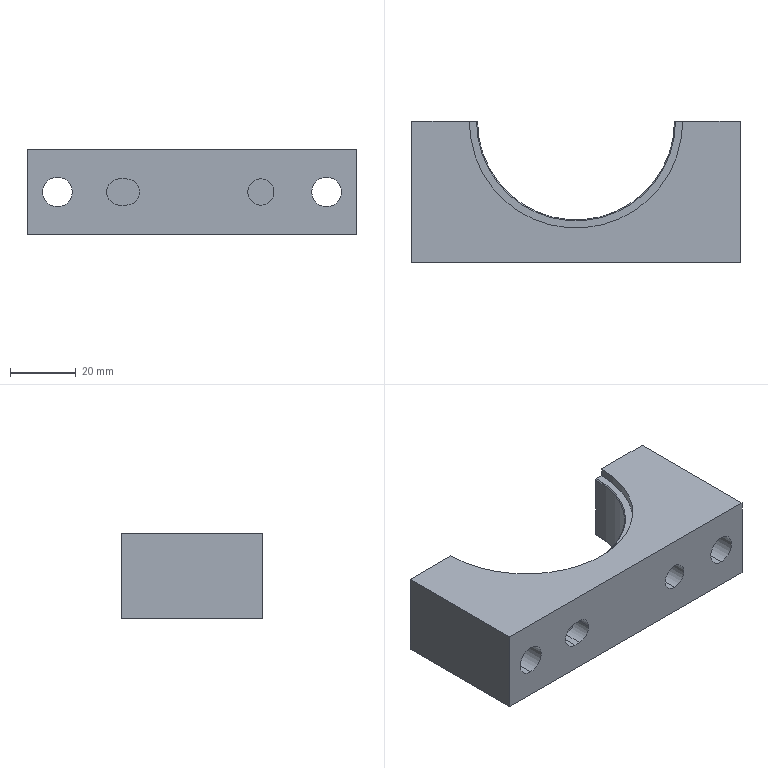Part | SolidWorks | features HoleWzd 3, ICE 3, Chamfer 1, Extrusion 1 | 1 solid | 30 faces | box 100 x 43 x 26 mm | volume 67587 mm3 | cylinder 14 | plane 14 | cone 2 | commonest cylinder face diameters 8 x5 9 x4 4 x2 65 x2 60 x1
STEP:
#1=CARTESIAN_POINT('',(-16.,-37.,13.));
#2=VERTEX_POINT('',#1);
#3=CARTESIAN_POINT('',(-20.,-37.,17.));
#4=VERTEX_POINT('',#3);
#5=CARTESIAN_POINT('',(-20.,-37.,13.));
#6=DIRECTION('',(0.,-1.,0.));
#7=DIRECTION('',(1.,0.,0.));
#8=AXIS2_PLACEMENT_3D('',#5,#6,#7);
#9=CIRCLE('',#8,4.);
#10=EDGE_CURVE('',#2,#4,#9,.T.);
#11=ORIENTED_EDGE('',*,*,#10,.F.);
#12=CARTESIAN_POINT('',(-16.,-43.,13.));
#13=VERTEX_POINT('',#12);
#14=CARTESIAN_POINT('',(-16.,-37.,13.));
#15=DIRECTION('',(0.,-1.,0.));
#16=VECTOR('',#15,1000.);
#17=LINE('',#14,#16);
#18=EDGE_CURVE('',#2,#13,#17,.T.);
#19=ORIENTED_EDGE('',*,*,#18,.T.);
#20=CARTESIAN_POINT('',(-20.,-43.,17.));
#21=VERTEX_POINT('',#20);
#22=CARTESIAN_POINT('',(-20.,-43.,13.));
#23=DIRECTION('',(0.,-1.,0.));
#24=DIRECTION('',(1.,0.,0.));
#25=AXIS2_PLACEMENT_3D('',#22,#23,#24);
#26=CIRCLE('',#25,4.);
#27=EDGE_CURVE('',#13,#21,#26,.T.);
#28=ORIENTED_EDGE('',*,*,#27,.T.);
#29=CARTESIAN_POINT('',(-20.,-37.,17.));
#30=DIRECTION('',(0.,-1.,0.));
#31=VECTOR('',#30,1000.);
#32=LINE('',#29,#31);
#33=EDGE_CURVE('',#4,#21,#32,.T.);
#34=ORIENTED_EDGE('',*,*,#33,.F.);
#35=EDGE_LOOP('',(#11,#19,#28,#34));
#36=FACE_OUTER_BOUND('',#35,.T.);
#37=CARTESIAN_POINT('',(-20.,-37.,13.));
#38=DIRECTION('',(0.,-1.,0.));
#39=DIRECTION('',(1.,0.,0.));
#40=AXIS2_PLACEMENT_3D('',#37,#38,#39);
#41=CYLINDRICAL_SURFACE('',#40,4.);
#42=ADVANCED_FACE('',(#36),#41,.F.);
#43=CARTESIAN_POINT('',(21.,-37.,17.));
#44=VERTEX_POINT('',#43);
#45=CARTESIAN_POINT('',(21.,-37.,9.));
#46=VERTEX_POINT('',#45);
#47=CARTESIAN_POINT('',(21.,-37.,13.));
#48=DIRECTION('',(0.,-1.,0.));
#49=DIRECTION('',(0.,0.,-1.));
#50=AXIS2_PLACEMENT_3D('',#47,#48,#49);
#51=CIRCLE('',#50,4.);
#52=EDGE_CURVE('',#44,#46,#51,.T.);
#53=ORIENTED_EDGE('',*,*,#52,.F.);
#54=CARTESIAN_POINT('',(21.,-43.,17.));
#55=VERTEX_POINT('',#54);
#56=CARTESIAN_POINT('',(21.,-43.,17.));
#57=DIRECTION('',(0.,-1.,0.));
#58=VECTOR('',#57,1000.);
#59=LINE('',#56,#58);
#60=EDGE_CURVE('',#44,#55,#59,.T.);
#61=ORIENTED_EDGE('',*,*,#60,.T.);
#62=CARTESIAN_POINT('',(21.,-43.,9.));
#63=VERTEX_POINT('',#62);
#64=CARTESIAN_POINT('',(21.,-43.,13.));
#65=DIRECTION('',(0.,-1.,0.));
#66=DIRECTION('',(0.,0.,-1.));
#67=AXIS2_PLACEMENT_3D('',#64,#65,#66);
#68=CIRCLE('',#67,4.);
#69=EDGE_CURVE('',#55,#63,#68,.T.);
#70=ORIENTED_EDGE('',*,*,#69,.T.);
#71=CARTESIAN_POINT('',(21.,-43.,9.));
#72=DIRECTION('',(0.,-1.,0.));
#73=VECTOR('',#72,1000.);
#74=LINE('',#71,#73);
#75=EDGE_CURVE('',#46,#63,#74,.T.);
#76=ORIENTED_EDGE('',*,*,#75,.F.);
#77=EDGE_LOOP('',(#53,#61,#70,#76));
#78=FACE_OUTER_BOUND('',#77,.T.);
#79=CARTESIAN_POINT('',(21.,-43.,13.));
#80=DIRECTION('',(0.,-1.,0.));
#81=DIRECTION('',(0.,0.,-1.));
#82=AXIS2_PLACEMENT_3D('',#79,#80,#81);
#83=CYLINDRICAL_SURFACE('',#82,4.);
#84=ADVANCED_FACE('',(#78),#83,.F.);
#85=CARTESIAN_POINT('',(0.,-34.,11.));
#86=VERTEX_POINT('',#85);
#87=CARTESIAN_POINT('',(0.,-34.,15.));
#88=VERTEX_POINT('',#87);
#89=CARTESIAN_POINT('',(0.,-34.,13.));
#90=DIRECTION('',(0.,1.,0.));
#91=DIRECTION('',(0.,0.,1.));
#92=AXIS2_PLACEMENT_3D('',#89,#90,#91);
#93=CIRCLE('',#92,2.);
#94=EDGE_CURVE('',#86,#88,#93,.T.);
#95=ORIENTED_EDGE('',*,*,#94,.F.);
#96=CARTESIAN_POINT('',(0.,-30.,11.));
#97=VERTEX_POINT('',#96);
#98=CARTESIAN_POINT('',(0.,0.,11.));
#99=DIRECTION('',(0.,1.,0.));
#100=VECTOR('',#99,1000.);
#101=LINE('',#98,#100);
#102=EDGE_CURVE('',#86,#97,#101,.T.);
#103=ORIENTED_EDGE('',*,*,#102,.T.);
#104=CARTESIAN_POINT('',(0.,-30.,15.));
#105=VERTEX_POINT('',#104);
#106=CARTESIAN_POINT('',(0.,-30.,15.));
#107=CARTESIAN_POINT('',(-0.1322,-30.,15.));
#108=CARTESIAN_POINT('',(-0.2622,-29.999,14.987));
#109=CARTESIAN_POINT('',(-0.5178,-29.996,14.936));
#110=CARTESIAN_POINT('',(-0.6449,-29.993,14.898));
#111=CARTESIAN_POINT('',(-0.8871,-29.987,14.797));
#112=CARTESIAN_POINT('',(-1.002,-29.983,14.736));
#113=CARTESIAN_POINT('',(-1.219,-29.975,14.591));
#114=CARTESIAN_POINT('',(-1.322,-29.971,14.506));
#115=CARTESIAN_POINT('',(-1.599,-29.958,14.229));
#116=CARTESIAN_POINT('',(-1.748,-29.949,14.006));
#117=CARTESIAN_POINT('',(-1.947,-29.937,13.525));
#118=CARTESIAN_POINT('',(-2.,-29.933,13.262));
#119=CARTESIAN_POINT('',(-2.,-29.933,12.87));
#120=CARTESIAN_POINT('',(-1.987,-29.934,12.738));
#121=CARTESIAN_POINT('',(-1.936,-29.937,12.481));
#122=CARTESIAN_POINT('',(-1.898,-29.94,12.356));
#123=CARTESIAN_POINT('',(-1.798,-29.946,12.114));
#124=CARTESIAN_POINT('',(-1.735,-29.95,11.997));
#125=CARTESIAN_POINT('',(-1.591,-29.958,11.78));
#126=CARTESIAN_POINT('',(-1.508,-29.962,11.679));
#127=CARTESIAN_POINT('',(-1.321,-29.971,11.493));
#128=CARTESIAN_POINT('',(-1.22,-29.975,11.41));
#129=CARTESIAN_POINT('',(-1.003,-29.983,11.265));
#130=CARTESIAN_POINT('',(-0.8865,-29.987,11.202));
#131=CARTESIAN_POINT('',(-0.6442,-29.993,11.102));
#132=CARTESIAN_POINT('',(-0.5195,-29.996,11.064));
#133=CARTESIAN_POINT('',(-0.2631,-29.999,11.013));
#134=CARTESIAN_POINT('',(-0.1305,-30.,11.));
#135=CARTESIAN_POINT('',(0.,-30.,11.));
#136=B_SPLINE_CURVE_WITH_KNOTS('',3,(#106,#107,#108,#109,#110,#111,#112,#113,#114,#115,#116,#117,#118,#119,#120,#121,#122,#123,#124,#125,#126,#127,#128,#129,#130,#131,#132,#133,#134,#135),.UNSPECIFIED.,.F.,.F.,(4,2,2,2,2,2,2,2,2,2,2,2,2,2,4),(0.,0.0003909,0.0007818,0.001173,0.001564,0.002345,0.003127,0.003518,0.003909,0.0043,0.004691,0.005082,0.005473,0.005864,0.006255),.UNSPECIFIED.);
#137=EDGE_CURVE('',#105,#97,#136,.T.);
#138=ORIENTED_EDGE('',*,*,#137,.F.);
#139=CARTESIAN_POINT('',(0.,0.,15.));
#140=DIRECTION('',(0.,1.,0.));
#141=VECTOR('',#140,1000.);
#142=LINE('',#139,#141);
#143=EDGE_CURVE('',#88,#105,#142,.T.);
#144=ORIENTED_EDGE('',*,*,#143,.F.);
#145=EDGE_LOOP('',(#95,#103,#138,#144));
#146=FACE_OUTER_BOUND('',#145,.T.);
#147=CARTESIAN_POINT('',(0.,0.,13.));
#148=DIRECTION('',(0.,1.,0.));
#149=DIRECTION('',(0.,0.,1.));
#150=AXIS2_PLACEMENT_3D('',#147,#148,#149);
#151=CYLINDRICAL_SURFACE('',#150,2.);
#152=ADVANCED_FACE('',(#146),#151,.F.);
#153=CARTESIAN_POINT('',(-41.,-43.,8.5));
#154=VERTEX_POINT('',#153);
#155=CARTESIAN_POINT('',(-41.,-43.,17.5));
#156=VERTEX_POINT('',#155);
#157=CARTESIAN_POINT('',(-41.,-43.,13.));
#158=DIRECTION('',(0.,1.,0.));
#159=DIRECTION('',(0.,0.,1.));
#160=AXIS2_PLACEMENT_3D('',#157,#158,#159);
#161=CIRCLE('',#160,4.5);
#162=EDGE_CURVE('',#154,#156,#161,.T.);
#163=ORIENTED_EDGE('',*,*,#162,.F.);
#164=CARTESIAN_POINT('',(-41.,0.,8.5));
#165=VERTEX_POINT('',#164);
#166=CARTESIAN_POINT('',(-41.,0.,8.5));
#167=DIRECTION('',(0.,1.,0.));
#168=VECTOR('',#167,1000.);
#169=LINE('',#166,#168);
#170=EDGE_CURVE('',#154,#165,#169,.T.);
#171=ORIENTED_EDGE('',*,*,#170,.T.);
#172=CARTESIAN_POINT('',(-41.,0.,17.5));
#173=VERTEX_POINT('',#172);
#174=CARTESIAN_POINT('',(-41.,0.,13.));
#175=DIRECTION('',(0.,1.,0.));
#176=DIRECTION('',(0.,0.,1.));
#177=AXIS2_PLACEMENT_3D('',#174,#175,#176);
#178=CIRCLE('',#177,4.5);
#179=EDGE_CURVE('',#165,#173,#178,.T.);
#180=ORIENTED_EDGE('',*,*,#179,.T.);
#181=CARTESIAN_POINT('',(-41.,0.,17.5));
#182=DIRECTION('',(0.,1.,0.));
#183=VECTOR('',#182,1000.);
#184=LINE('',#181,#183);
#185=EDGE_CURVE('',#156,#173,#184,.T.);
#186=ORIENTED_EDGE('',*,*,#185,.F.);
#187=EDGE_LOOP('',(#163,#171,#180,#186));
#188=FACE_OUTER_BOUND('',#187,.T.);
#189=CARTESIAN_POINT('',(-41.,0.,13.));
#190=DIRECTION('',(0.,1.,0.));
#191=DIRECTION('',(0.,0.,1.));
#192=AXIS2_PLACEMENT_3D('',#189,#190,#191);
#193=CYLINDRICAL_SURFACE('',#192,4.5);
#194=ADVANCED_FACE('',(#188),#193,.F.);
#195=CARTESIAN_POINT('',(41.,-43.,8.5));
#196=VERTEX_POINT('',#195);
#197=CARTESIAN_POINT('',(41.,-43.,17.5));
#198=VERTEX_POINT('',#197);
#199=CARTESIAN_POINT('',(41.,-43.,13.));
#200=DIRECTION('',(0.,1.,0.));
#201=DIRECTION('',(0.,0.,1.));
#202=AXIS2_PLACEMENT_3D('',#199,#200,#201);
#203=CIRCLE('',#202,4.5);
#204=EDGE_CURVE('',#196,#198,#203,.T.);
#205=ORIENTED_EDGE('',*,*,#204,.F.);
#206=CARTESIAN_POINT('',(41.,0.,8.5));
#207=VERTEX_POINT('',#206);
#208=CARTESIAN_POINT('',(41.,0.,8.5));
#209=DIRECTION('',(0.,1.,0.));
#210=VECTOR('',#209,1000.);
#211=LINE('',#208,#210);
#212=EDGE_CURVE('',#196,#207,#211,.T.);
#213=ORIENTED_EDGE('',*,*,#212,.T.);
#214=CARTESIAN_POINT('',(41.,0.,17.5));
#215=VERTEX_POINT('',#214);
#216=CARTESIAN_POINT('',(41.,0.,13.));
#217=DIRECTION('',(0.,1.,0.));
#218=DIRECTION('',(0.,0.,1.));
#219=AXIS2_PLACEMENT_3D('',#216,#217,#218);
#220=CIRCLE('',#219,4.5);
#221=EDGE_CURVE('',#207,#215,#220,.T.);
#222=ORIENTED_EDGE('',*,*,#221,.T.);
#223=CARTESIAN_POINT('',(41.,0.,17.5));
#224=DIRECTION('',(0.,1.,0.));
#225=VECTOR('',#224,1000.);
#226=LINE('',#223,#225);
#227=EDGE_CURVE('',#198,#215,#226,.T.);
#228=ORIENTED_EDGE('',*,*,#227,.F.);
#229=EDGE_LOOP('',(#205,#213,#222,#228));
#230=FACE_OUTER_BOUND('',#229,.T.);
#231=CARTESIAN_POINT('',(41.,0.,13.));
#232=DIRECTION('',(0.,1.,0.));
#233=DIRECTION('',(0.,0.,1.));
#234=AXIS2_PLACEMENT_3D('',#231,#232,#233);
#235=CYLINDRICAL_SURFACE('',#234,4.5);
#236=ADVANCED_FACE('',(#230),#235,.F.);
#237=ORIENTED_EDGE('',*,*,#137,.T.);
#238=CARTESIAN_POINT('',(0.,-30.,11.));
#239=CARTESIAN_POINT('',(0.261,-30.,11.));
#240=CARTESIAN_POINT('',(0.5242,-29.996,11.052));
#241=CARTESIAN_POINT('',(1.006,-29.984,11.252));
#242=CARTESIAN_POINT('',(1.229,-29.975,11.401));
#243=CARTESIAN_POINT('',(1.505,-29.962,11.677));
#244=CARTESIAN_POINT('',(1.59,-29.958,11.78));
#245=CARTESIAN_POINT('',(1.735,-29.95,11.997));
#246=CARTESIAN_POINT('',(1.797,-29.946,12.112));
#247=CARTESIAN_POINT('',(1.897,-29.94,12.354));
#248=CARTESIAN_POINT('',(1.936,-29.937,12.481));
#249=CARTESIAN_POINT('',(1.987,-29.934,12.737));
#250=CARTESIAN_POINT('',(2.,-29.933,12.866));
#251=CARTESIAN_POINT('',(2.,-29.933,13.13));
#252=CARTESIAN_POINT('',(1.987,-29.934,13.261));
#253=CARTESIAN_POINT('',(1.937,-29.937,13.516));
#254=CARTESIAN_POINT('',(1.898,-29.94,13.643));
#255=CARTESIAN_POINT('',(1.798,-29.946,13.886));
#256=CARTESIAN_POINT('',(1.737,-29.95,14.001));
#257=CARTESIAN_POINT('',(1.592,-29.958,14.218));
#258=CARTESIAN_POINT('',(1.507,-29.962,14.321));
#259=CARTESIAN_POINT('',(1.323,-29.971,14.506));
#260=CARTESIAN_POINT('',(1.222,-29.975,14.588));
#261=CARTESIAN_POINT('',(1.004,-29.983,14.735));
#262=CARTESIAN_POINT('',(0.8877,-29.987,14.797));
#263=CARTESIAN_POINT('',(0.5269,-29.996,14.947));
#264=CARTESIAN_POINT('',(0.2643,-30.,15.));
#265=CARTESIAN_POINT('',(0.,-30.,15.));
#266=B_SPLINE_CURVE_WITH_KNOTS('',3,(#238,#239,#240,#241,#242,#243,#244,#245,#246,#247,#248,#249,#250,#251,#252,#253,#254,#255,#256,#257,#258,#259,#260,#261,#262,#263,#264,#265),.UNSPECIFIED.,.F.,.F.,(4,2,2,2,2,2,2,2,2,2,2,2,2,4),(0.006255,0.007036,0.007818,0.008209,0.0086,0.00899,0.009381,0.009772,0.01016,0.01055,0.01094,0.01134,0.01173,0.01251),.UNSPECIFIED.);
#267=EDGE_CURVE('',#97,#105,#266,.T.);
#268=ORIENTED_EDGE('',*,*,#267,.T.);
#269=EDGE_LOOP('',(#237,#268));
#270=FACE_BOUND('',#269,.T.);
#271=CARTESIAN_POINT('',(30.,0.,23.2));
#272=VERTEX_POINT('',#271);
#273=CARTESIAN_POINT('',(30.,0.,2.8));
#274=VERTEX_POINT('',#273);
#275=CARTESIAN_POINT('',(30.,0.,26.));
#276=DIRECTION('',(0.,0.,-1.));
#277=VECTOR('',#276,1000.);
#278=LINE('',#275,#277);
#279=EDGE_CURVE('',#272,#274,#278,.T.);
#280=ORIENTED_EDGE('',*,*,#279,.T.);
#281=CARTESIAN_POINT('',(-30.,0.,2.8));
#282=VERTEX_POINT('',#281);
#283=CARTESIAN_POINT('',(0.,0.,2.8));
#284=DIRECTION('',(0.,0.,-1.));
#285=DIRECTION('',(-1.,0.,0.));
#286=AXIS2_PLACEMENT_3D('',#283,#284,#285);
#287=CIRCLE('',#286,30.);
#288=EDGE_CURVE('',#274,#282,#287,.T.);
#289=ORIENTED_EDGE('',*,*,#288,.T.);
#290=CARTESIAN_POINT('',(-30.,0.,23.2));
#291=VERTEX_POINT('',#290);
#292=CARTESIAN_POINT('',(-30.,0.,26.));
#293=DIRECTION('',(0.,0.,-1.));
#294=VECTOR('',#293,1000.);
#295=LINE('',#292,#294);
#296=EDGE_CURVE('',#291,#282,#295,.T.);
#297=ORIENTED_EDGE('',*,*,#296,.F.);
#298=CARTESIAN_POINT('',(0.,0.,23.2));
#299=DIRECTION('',(0.,0.,1.));
#300=DIRECTION('',(1.,0.,0.));
#301=AXIS2_PLACEMENT_3D('',#298,#299,#300);
#302=CIRCLE('',#301,30.);
#303=EDGE_CURVE('',#291,#272,#302,.T.);
#304=ORIENTED_EDGE('',*,*,#303,.T.);
#305=EDGE_LOOP('',(#280,#289,#297,#304));
#306=FACE_OUTER_BOUND('',#305,.T.);
#307=CARTESIAN_POINT('',(0.,0.,26.));
#308=DIRECTION('',(0.,0.,-1.));
#309=DIRECTION('',(-1.,0.,0.));
#310=AXIS2_PLACEMENT_3D('',#307,#308,#309);
#311=CYLINDRICAL_SURFACE('',#310,30.);
#312=ADVANCED_FACE('',(#270,#306),#311,.F.);
#313=CARTESIAN_POINT('',(-41.,0.,13.));
#314=DIRECTION('',(0.,1.,0.));
#315=DIRECTION('',(0.,0.,1.));
#316=AXIS2_PLACEMENT_3D('',#313,#314,#315);
#317=CIRCLE('',#316,4.5);
#318=EDGE_CURVE('',#173,#165,#317,.T.);
#319=ORIENTED_EDGE('',*,*,#318,.F.);
#320=ORIENTED_EDGE('',*,*,#179,.F.);
#321=EDGE_LOOP('',(#319,#320));
#322=FACE_BOUND('',#321,.T.);
#323=ORIENTED_EDGE('',*,*,#296,.T.);
#324=CARTESIAN_POINT('',(-30.3,0.,2.5));
#325=VERTEX_POINT('',#324);
#326=CARTESIAN_POINT('',(0.,0.,32.8));
#327=DIRECTION('',(-0.7071,0.,-0.7071));
#328=VECTOR('',#327,1000.);
#329=LINE('',#326,#328);
#330=EDGE_CURVE('',#282,#325,#329,.T.);
#331=ORIENTED_EDGE('',*,*,#330,.T.);
#332=CARTESIAN_POINT('',(-32.5,0.,2.5));
#333=VERTEX_POINT('',#332);
#334=CARTESIAN_POINT('',(-50.,0.,2.5));
#335=DIRECTION('',(1.,0.,0.));
#336=VECTOR('',#335,1000.);
#337=LINE('',#334,#336);
#338=EDGE_CURVE('',#333,#325,#337,.T.);
#339=ORIENTED_EDGE('',*,*,#338,.F.);
#340=CARTESIAN_POINT('',(-32.5,0.,0.));
#341=VERTEX_POINT('',#340);
#342=CARTESIAN_POINT('',(-32.5,0.,2.5));
#343=DIRECTION('',(0.,0.,-1.));
#344=VECTOR('',#343,1000.);
#345=LINE('',#342,#344);
#346=EDGE_CURVE('',#333,#341,#345,.T.);
#347=ORIENTED_EDGE('',*,*,#346,.T.);
#348=CARTESIAN_POINT('',(-50.,0.,0.));
#349=VERTEX_POINT('',#348);
#350=CARTESIAN_POINT('',(-50.,0.,0.));
#351=DIRECTION('',(-1.,0.,0.));
#352=VECTOR('',#351,1000.);
#353=LINE('',#350,#352);
#354=EDGE_CURVE('',#341,#349,#353,.T.);
#355=ORIENTED_EDGE('',*,*,#354,.T.);
#356=CARTESIAN_POINT('',(-50.,0.,26.));
#357=VERTEX_POINT('',#356);
#358=CARTESIAN_POINT('',(-50.,0.,26.));
#359=DIRECTION('',(0.,0.,-1.));
#360=VECTOR('',#359,1000.);
#361=LINE('',#358,#360);
#362=EDGE_CURVE('',#357,#349,#361,.T.);
#363=ORIENTED_EDGE('',*,*,#362,.F.);
#364=CARTESIAN_POINT('',(-32.5,0.,26.));
#365=VERTEX_POINT('',#364);
#366=CARTESIAN_POINT('',(-50.,0.,26.));
#367=DIRECTION('',(-1.,0.,0.));
#368=VECTOR('',#367,1000.);
#369=LINE('',#366,#368);
#370=EDGE_CURVE('',#365,#357,#369,.T.);
#371=ORIENTED_EDGE('',*,*,#370,.F.);
#372=CARTESIAN_POINT('',(-32.5,0.,23.5));
#373=VERTEX_POINT('',#372);
#374=CARTESIAN_POINT('',(-32.5,0.,23.5));
#375=DIRECTION('',(0.,0.,-1.));
#376=VECTOR('',#375,1000.);
#377=LINE('',#374,#376);
#378=EDGE_CURVE('',#365,#373,#377,.T.);
#379=ORIENTED_EDGE('',*,*,#378,.T.);
#380=CARTESIAN_POINT('',(-30.3,0.,23.5));
#381=VERTEX_POINT('',#380);
#382=CARTESIAN_POINT('',(-50.,0.,23.5));
#383=DIRECTION('',(-1.,0.,0.));
#384=VECTOR('',#383,1000.);
#385=LINE('',#382,#384);
#386=EDGE_CURVE('',#381,#373,#385,.T.);
#387=ORIENTED_EDGE('',*,*,#386,.F.);
#388=CARTESIAN_POINT('',(0.,0.,-6.8));
#389=DIRECTION('',(0.7071,0.,-0.7071));
#390=VECTOR('',#389,1000.);
#391=LINE('',#388,#390);
#392=EDGE_CURVE('',#381,#291,#391,.T.);
#393=ORIENTED_EDGE('',*,*,#392,.T.);
#394=EDGE_LOOP('',(#323,#331,#339,#347,#355,#363,#371,#379,#387,#393));
#395=FACE_OUTER_BOUND('',#394,.T.);
#396=CARTESIAN_POINT('',(-50.,0.,26.));
#397=DIRECTION('',(0.,-1.,0.));
#398=DIRECTION('',(1.,0.,0.));
#399=AXIS2_PLACEMENT_3D('',#396,#397,#398);
#400=PLANE('',#399);
#401=ADVANCED_FACE('',(#322,#395),#400,.F.);
#402=CARTESIAN_POINT('',(-50.,-43.,0.));
#403=VERTEX_POINT('',#402);
#404=CARTESIAN_POINT('',(-50.,-43.,0.));
#405=DIRECTION('',(0.,-1.,0.));
#406=VECTOR('',#405,1000.);
#407=LINE('',#404,#406);
#408=EDGE_CURVE('',#349,#403,#407,.T.);
#409=ORIENTED_EDGE('',*,*,#408,.T.);
#410=CARTESIAN_POINT('',(-50.,-43.,26.));
#411=VERTEX_POINT('',#410);
#412=CARTESIAN_POINT('',(-50.,-43.,26.));
#413=DIRECTION('',(0.,0.,-1.));
#414=VECTOR('',#413,1000.);
#415=LINE('',#412,#414);
#416=EDGE_CURVE('',#411,#403,#415,.T.);
#417=ORIENTED_EDGE('',*,*,#416,.F.);
#418=CARTESIAN_POINT('',(-50.,-43.,26.));
#419=DIRECTION('',(0.,-1.,0.));
#420=VECTOR('',#419,1000.);
#421=LINE('',#418,#420);
#422=EDGE_CURVE('',#357,#411,#421,.T.);
#423=ORIENTED_EDGE('',*,*,#422,.F.);
#424=ORIENTED_EDGE('',*,*,#362,.T.);
#425=EDGE_LOOP('',(#409,#417,#423,#424));
#426=FACE_OUTER_BOUND('',#425,.T.);
#427=CARTESIAN_POINT('',(-50.,-43.,26.));
#428=DIRECTION('',(1.,0.,0.));
#429=DIRECTION('',(0.,0.,-1.));
#430=AXIS2_PLACEMENT_3D('',#427,#428,#429);
#431=PLANE('',#430);
#432=ADVANCED_FACE('',(#426),#431,.F.);
#433=CARTESIAN_POINT('',(-22.,-43.,17.));
#434=VERTEX_POINT('',#433);
#435=CARTESIAN_POINT('',(-22.,-43.,9.));
#436=VERTEX_POINT('',#435);
#437=CARTESIAN_POINT('',(-22.,-43.,13.));
#438=DIRECTION('',(0.,-1.,0.));
#439=DIRECTION('',(1.,0.,0.));
#440=AXIS2_PLACEMENT_3D('',#437,#438,#439);
#441=CIRCLE('',#440,4.);
#442=EDGE_CURVE('',#434,#436,#441,.T.);
#443=ORIENTED_EDGE('',*,*,#442,.F.);
#444=CARTESIAN_POINT('',(0.,-43.,17.));
#445=DIRECTION('',(-1.,0.,0.));
#446=VECTOR('',#445,1000.);
#447=LINE('',#444,#446);
#448=EDGE_CURVE('',#21,#434,#447,.T.);
#449=ORIENTED_EDGE('',*,*,#448,.F.);
#450=ORIENTED_EDGE('',*,*,#27,.F.);
#451=CARTESIAN_POINT('',(-20.,-43.,9.));
#452=VERTEX_POINT('',#451);
#453=CARTESIAN_POINT('',(-20.,-43.,13.));
#454=DIRECTION('',(0.,-1.,0.));
#455=DIRECTION('',(1.,0.,0.));
#456=AXIS2_PLACEMENT_3D('',#453,#454,#455);
#457=CIRCLE('',#456,4.);
#458=EDGE_CURVE('',#452,#13,#457,.T.);
#459=ORIENTED_EDGE('',*,*,#458,.F.);
#460=CARTESIAN_POINT('',(0.,-43.,9.));
#461=DIRECTION('',(-1.,0.,0.));
#462=VECTOR('',#461,1000.);
#463=LINE('',#460,#462);
#464=EDGE_CURVE('',#452,#436,#463,.T.);
#465=ORIENTED_EDGE('',*,*,#464,.T.);
#466=EDGE_LOOP('',(#443,#449,#450,#459,#465));
#467=FACE_BOUND('',#466,.T.);
#468=CARTESIAN_POINT('',(21.,-43.,13.));
#469=DIRECTION('',(0.,-1.,0.));
#470=DIRECTION('',(0.,0.,-1.));
#471=AXIS2_PLACEMENT_3D('',#468,#469,#470);
#472=CIRCLE('',#471,4.);
#473=EDGE_CURVE('',#63,#55,#472,.T.);
#474=ORIENTED_EDGE('',*,*,#473,.F.);
#475=ORIENTED_EDGE('',*,*,#69,.F.);
#476=EDGE_LOOP('',(#474,#475));
#477=FACE_BOUND('',#476,.T.);
#478=CARTESIAN_POINT('',(-41.,-43.,13.));
#479=DIRECTION('',(0.,1.,0.));
#480=DIRECTION('',(0.,0.,1.));
#481=AXIS2_PLACEMENT_3D('',#478,#479,#480);
#482=CIRCLE('',#481,4.5);
#483=EDGE_CURVE('',#156,#154,#482,.T.);
#484=ORIENTED_EDGE('',*,*,#483,.T.);
#485=ORIENTED_EDGE('',*,*,#162,.T.);
#486=EDGE_LOOP('',(#484,#485));
#487=FACE_BOUND('',#486,.T.);
#488=CARTESIAN_POINT('',(41.,-43.,13.));
#489=DIRECTION('',(0.,1.,0.));
#490=DIRECTION('',(0.,0.,1.));
#491=AXIS2_PLACEMENT_3D('',#488,#489,#490);
#492=CIRCLE('',#491,4.5);
#493=EDGE_CURVE('',#198,#196,#492,.T.);
#494=ORIENTED_EDGE('',*,*,#493,.T.);
#495=ORIENTED_EDGE('',*,*,#204,.T.);
#496=EDGE_LOOP('',(#494,#495));
#497=FACE_BOUND('',#496,.T.);
#498=CARTESIAN_POINT('',(50.,-43.,0.));
#499=VERTEX_POINT('',#498);
#500=CARTESIAN_POINT('',(-50.,-43.,0.));
#501=DIRECTION('',(1.,0.,0.));
#502=VECTOR('',#501,1000.);
#503=LINE('',#500,#502);
#504=EDGE_CURVE('',#403,#499,#503,.T.);
#505=ORIENTED_EDGE('',*,*,#504,.T.);
#506=CARTESIAN_POINT('',(50.,-43.,26.));
#507=VERTEX_POINT('',#506);
#508=CARTESIAN_POINT('',(50.,-43.,26.));
#509=DIRECTION('',(0.,0.,-1.));
#510=VECTOR('',#509,1000.);
#511=LINE('',#508,#510);
#512=EDGE_CURVE('',#507,#499,#511,.T.);
#513=ORIENTED_EDGE('',*,*,#512,.F.);
#514=CARTESIAN_POINT('',(-50.,-43.,26.));
#515=DIRECTION('',(1.,0.,0.));
#516=VECTOR('',#515,1000.);
#517=LINE('',#514,#516);
#518=EDGE_CURVE('',#411,#507,#517,.T.);
#519=ORIENTED_EDGE('',*,*,#518,.F.);
#520=ORIENTED_EDGE('',*,*,#416,.T.);
#521=EDGE_LOOP('',(#505,#513,#519,#520));
#522=FACE_OUTER_BOUND('',#521,.T.);
#523=CARTESIAN_POINT('',(-50.,-43.,26.));
#524=DIRECTION('',(0.,1.,0.));
#525=DIRECTION('',(-1.,0.,0.));
#526=AXIS2_PLACEMENT_3D('',#523,#524,#525);
#527=PLANE('',#526);
#528=ADVANCED_FACE('',(#467,#477,#487,#497,#522),#527,.F.);
#529=CARTESIAN_POINT('',(50.,0.,0.));
#530=VERTEX_POINT('',#529);
#531=CARTESIAN_POINT('',(50.,-43.,0.));
#532=DIRECTION('',(0.,1.,0.));
#533=VECTOR('',#532,1000.);
#534=LINE('',#531,#533);
#535=EDGE_CURVE('',#499,#530,#534,.T.);
#536=ORIENTED_EDGE('',*,*,#535,.T.);
#537=CARTESIAN_POINT('',(50.,0.,26.));
#538=VERTEX_POINT('',#537);
#539=CARTESIAN_POINT('',(50.,0.,26.));
#540=DIRECTION('',(0.,0.,-1.));
#541=VECTOR('',#540,1000.);
#542=LINE('',#539,#541);
#543=EDGE_CURVE('',#538,#530,#542,.T.);
#544=ORIENTED_EDGE('',*,*,#543,.F.);
#545=CARTESIAN_POINT('',(50.,-43.,26.));
#546=DIRECTION('',(0.,1.,0.));
#547=VECTOR('',#546,1000.);
#548=LINE('',#545,#547);
#549=EDGE_CURVE('',#507,#538,#548,.T.);
#550=ORIENTED_EDGE('',*,*,#549,.F.);
#551=ORIENTED_EDGE('',*,*,#512,.T.);
#552=EDGE_LOOP('',(#536,#544,#550,#551));
#553=FACE_OUTER_BOUND('',#552,.T.);
#554=CARTESIAN_POINT('',(50.,-43.,26.));
#555=DIRECTION('',(-1.,0.,0.));
#556=DIRECTION('',(0.,-1.,0.));
#557=AXIS2_PLACEMENT_3D('',#554,#555,#556);
#558=PLANE('',#557);
#559=ADVANCED_FACE('',(#553),#558,.F.);
#560=CARTESIAN_POINT('',(41.,0.,13.));
#561=DIRECTION('',(0.,1.,0.));
#562=DIRECTION('',(0.,0.,1.));
#563=AXIS2_PLACEMENT_3D('',#560,#561,#562);
#564=CIRCLE('',#563,4.5);
#565=EDGE_CURVE('',#215,#207,#564,.T.);
#566=ORIENTED_EDGE('',*,*,#565,.F.);
#567=ORIENTED_EDGE('',*,*,#221,.F.);
#568=EDGE_LOOP('',(#566,#567));
#569=FACE_BOUND('',#568,.T.);
#570=CARTESIAN_POINT('',(30.3,0.,2.5));
#571=VERTEX_POINT('',#570);
#572=CARTESIAN_POINT('',(32.5,0.,2.5));
#573=VERTEX_POINT('',#572);
#574=CARTESIAN_POINT('',(30.,0.,2.5));
#575=DIRECTION('',(1.,0.,0.));
#576=VECTOR('',#575,1000.);
#577=LINE('',#574,#576);
#578=EDGE_CURVE('',#571,#573,#577,.T.);
#579=ORIENTED_EDGE('',*,*,#578,.F.);
#580=CARTESIAN_POINT('',(0.,0.,32.8));
#581=DIRECTION('',(-0.7071,0.,0.7071));
#582=VECTOR('',#581,1000.);
#583=LINE('',#580,#582);
#584=EDGE_CURVE('',#571,#274,#583,.T.);
#585=ORIENTED_EDGE('',*,*,#584,.T.);
#586=ORIENTED_EDGE('',*,*,#279,.F.);
#587=CARTESIAN_POINT('',(30.3,0.,23.5));
#588=VERTEX_POINT('',#587);
#589=CARTESIAN_POINT('',(0.,0.,-6.8));
#590=DIRECTION('',(0.7071,0.,0.7071));
#591=VECTOR('',#590,1000.);
#592=LINE('',#589,#591);
#593=EDGE_CURVE('',#272,#588,#592,.T.);
#594=ORIENTED_EDGE('',*,*,#593,.T.);
#595=CARTESIAN_POINT('',(32.5,0.,23.5));
#596=VERTEX_POINT('',#595);
#597=CARTESIAN_POINT('',(30.,0.,23.5));
#598=DIRECTION('',(-1.,0.,0.));
#599=VECTOR('',#598,1000.);
#600=LINE('',#597,#599);
#601=EDGE_CURVE('',#596,#588,#600,.T.);
#602=ORIENTED_EDGE('',*,*,#601,.F.);
#603=CARTESIAN_POINT('',(32.5,0.,26.));
#604=VERTEX_POINT('',#603);
#605=CARTESIAN_POINT('',(32.5,0.,23.5));
#606=DIRECTION('',(0.,0.,1.));
#607=VECTOR('',#606,1000.);
#608=LINE('',#605,#607);
#609=EDGE_CURVE('',#596,#604,#608,.T.);
#610=ORIENTED_EDGE('',*,*,#609,.T.);
#611=CARTESIAN_POINT('',(30.,0.,26.));
#612=DIRECTION('',(-1.,0.,0.));
#613=VECTOR('',#612,1000.);
#614=LINE('',#611,#613);
#615=EDGE_CURVE('',#538,#604,#614,.T.);
#616=ORIENTED_EDGE('',*,*,#615,.F.);
#617=ORIENTED_EDGE('',*,*,#543,.T.);
#618=CARTESIAN_POINT('',(32.5,0.,0.));
#619=VERTEX_POINT('',#618);
#620=CARTESIAN_POINT('',(30.,0.,0.));
#621=DIRECTION('',(-1.,0.,0.));
#622=VECTOR('',#621,1000.);
#623=LINE('',#620,#622);
#624=EDGE_CURVE('',#530,#619,#623,.T.);
#625=ORIENTED_EDGE('',*,*,#624,.T.);
#626=CARTESIAN_POINT('',(32.5,0.,2.5));
#627=DIRECTION('',(0.,0.,1.));
#628=VECTOR('',#627,1000.);
#629=LINE('',#626,#628);
#630=EDGE_CURVE('',#619,#573,#629,.T.);
#631=ORIENTED_EDGE('',*,*,#630,.T.);
#632=EDGE_LOOP('',(#579,#585,#586,#594,#602,#610,#616,#617,#625,#631));
#633=FACE_OUTER_BOUND('',#632,.T.);
#634=CARTESIAN_POINT('',(30.,0.,26.));
#635=DIRECTION('',(0.,-1.,0.));
#636=DIRECTION('',(1.,0.,0.));
#637=AXIS2_PLACEMENT_3D('',#634,#635,#636);
#638=PLANE('',#637);
#639=ADVANCED_FACE('',(#569,#633),#638,.F.);
#640=CARTESIAN_POINT('',(0.,0.,26.));
#641=DIRECTION('',(0.,0.,1.));
#642=DIRECTION('',(1.,0.,0.));
#643=AXIS2_PLACEMENT_3D('',#640,#641,#642);
#644=CIRCLE('',#643,32.5);
#645=EDGE_CURVE('',#365,#604,#644,.T.);
#646=ORIENTED_EDGE('',*,*,#645,.F.);
#647=ORIENTED_EDGE('',*,*,#370,.T.);
#648=ORIENTED_EDGE('',*,*,#422,.T.);
#649=ORIENTED_EDGE('',*,*,#518,.T.);
#650=ORIENTED_EDGE('',*,*,#549,.T.);
#651=ORIENTED_EDGE('',*,*,#615,.T.);
#652=EDGE_LOOP('',(#646,#647,#648,#649,#650,#651));
#653=FACE_OUTER_BOUND('',#652,.T.);
#654=CARTESIAN_POINT('',(0.,0.,26.));
#655=DIRECTION('',(0.,0.,1.));
#656=DIRECTION('',(1.,0.,0.));
#657=AXIS2_PLACEMENT_3D('',#654,#655,#656);
#658=PLANE('',#657);
#659=ADVANCED_FACE('',(#653),#658,.T.);
#660=ORIENTED_EDGE('',*,*,#354,.F.);
#661=CARTESIAN_POINT('',(0.,0.,0.));
#662=DIRECTION('',(0.,0.,1.));
#663=DIRECTION('',(1.,0.,0.));
#664=AXIS2_PLACEMENT_3D('',#661,#662,#663);
#665=CIRCLE('',#664,32.5);
#666=EDGE_CURVE('',#341,#619,#665,.T.);
#667=ORIENTED_EDGE('',*,*,#666,.T.);
#668=ORIENTED_EDGE('',*,*,#624,.F.);
#669=ORIENTED_EDGE('',*,*,#535,.F.);
#670=ORIENTED_EDGE('',*,*,#504,.F.);
#671=ORIENTED_EDGE('',*,*,#408,.F.);
#672=EDGE_LOOP('',(#660,#667,#668,#669,#670,#671));
#673=FACE_OUTER_BOUND('',#672,.T.);
#674=CARTESIAN_POINT('',(0.,0.,0.));
#675=DIRECTION('',(0.,0.,1.));
#676=DIRECTION('',(1.,0.,0.));
#677=AXIS2_PLACEMENT_3D('',#674,#675,#676);
#678=PLANE('',#677);
#679=ADVANCED_FACE('',(#673),#678,.F.);
#680=ORIENTED_EDGE('',*,*,#601,.T.);
#681=CARTESIAN_POINT('',(0.,0.,23.5));
#682=DIRECTION('',(0.,0.,-1.));
#683=DIRECTION('',(1.,0.,0.));
#684=AXIS2_PLACEMENT_3D('',#681,#682,#683);
#685=CIRCLE('',#684,30.3);
#686=EDGE_CURVE('',#588,#381,#685,.T.);
#687=ORIENTED_EDGE('',*,*,#686,.T.);
#688=ORIENTED_EDGE('',*,*,#386,.T.);
#689=CARTESIAN_POINT('',(0.,0.,23.5));
#690=DIRECTION('',(0.,0.,1.));
#691=DIRECTION('',(1.,0.,0.));
#692=AXIS2_PLACEMENT_3D('',#689,#690,#691);
#693=CIRCLE('',#692,32.5);
#694=EDGE_CURVE('',#373,#596,#693,.T.);
#695=ORIENTED_EDGE('',*,*,#694,.T.);
#696=EDGE_LOOP('',(#680,#687,#688,#695));
#697=FACE_OUTER_BOUND('',#696,.T.);
#698=CARTESIAN_POINT('',(0.,0.,23.5));
#699=DIRECTION('',(0.,0.,1.));
#700=DIRECTION('',(1.,0.,0.));
#701=AXIS2_PLACEMENT_3D('',#698,#699,#700);
#702=PLANE('',#701);
#703=ADVANCED_FACE('',(#697),#702,.T.);
#704=ORIENTED_EDGE('',*,*,#645,.T.);
#705=ORIENTED_EDGE('',*,*,#609,.F.);
#706=ORIENTED_EDGE('',*,*,#694,.F.);
#707=ORIENTED_EDGE('',*,*,#378,.F.);
#708=EDGE_LOOP('',(#704,#705,#706,#707));
#709=FACE_OUTER_BOUND('',#708,.T.);
#710=CARTESIAN_POINT('',(0.,0.,23.5));
#711=DIRECTION('',(0.,0.,1.));
#712=DIRECTION('',(1.,0.,0.));
#713=AXIS2_PLACEMENT_3D('',#710,#711,#712);
#714=CYLINDRICAL_SURFACE('',#713,32.5);
#715=ADVANCED_FACE('',(#709),#714,.F.);
#716=ORIENTED_EDGE('',*,*,#338,.T.);
#717=CARTESIAN_POINT('',(0.,0.,2.5));
#718=DIRECTION('',(0.,0.,1.));
#719=DIRECTION('',(-1.,0.,0.));
#720=AXIS2_PLACEMENT_3D('',#717,#718,#719);
#721=CIRCLE('',#720,30.3);
#722=EDGE_CURVE('',#325,#571,#721,.T.);
#723=ORIENTED_EDGE('',*,*,#722,.T.);
#724=ORIENTED_EDGE('',*,*,#578,.T.);
#725=CARTESIAN_POINT('',(0.,0.,2.5));
#726=DIRECTION('',(0.,0.,-1.));
#727=DIRECTION('',(-1.,0.,0.));
#728=AXIS2_PLACEMENT_3D('',#725,#726,#727);
#729=CIRCLE('',#728,32.5);
#730=EDGE_CURVE('',#573,#333,#729,.T.);
#731=ORIENTED_EDGE('',*,*,#730,.T.);
#732=EDGE_LOOP('',(#716,#723,#724,#731));
#733=FACE_OUTER_BOUND('',#732,.T.);
#734=CARTESIAN_POINT('',(0.,0.,2.5));
#735=DIRECTION('',(0.,0.,-1.));
#736=DIRECTION('',(-1.,0.,0.));
#737=AXIS2_PLACEMENT_3D('',#734,#735,#736);
#738=PLANE('',#737);
#739=ADVANCED_FACE('',(#733),#738,.T.);
#740=ORIENTED_EDGE('',*,*,#730,.F.);
#741=ORIENTED_EDGE('',*,*,#630,.F.);
#742=ORIENTED_EDGE('',*,*,#666,.F.);
#743=ORIENTED_EDGE('',*,*,#346,.F.);
#744=EDGE_LOOP('',(#740,#741,#742,#743));
#745=FACE_OUTER_BOUND('',#744,.T.);
#746=CARTESIAN_POINT('',(0.,0.,2.5));
#747=DIRECTION('',(0.,0.,-1.));
#748=DIRECTION('',(-1.,0.,0.));
#749=AXIS2_PLACEMENT_3D('',#746,#747,#748);
#750=CYLINDRICAL_SURFACE('',#749,32.5);
#751=ADVANCED_FACE('',(#745),#750,.F.);
#752=ORIENTED_EDGE('',*,*,#330,.F.);
#753=ORIENTED_EDGE('',*,*,#288,.F.);
#754=ORIENTED_EDGE('',*,*,#584,.F.);
#755=ORIENTED_EDGE('',*,*,#722,.F.);
#756=EDGE_LOOP('',(#752,#753,#754,#755));
#757=FACE_OUTER_BOUND('',#756,.T.);
#758=CARTESIAN_POINT('',(0.,0.,2.5));
#759=DIRECTION('',(0.,0.,-1.));
#760=DIRECTION('',(-1.,0.,0.));
#761=AXIS2_PLACEMENT_3D('',#758,#759,#760);
#762=CONICAL_SURFACE('',#761,30.3,0.7854);
#763=ADVANCED_FACE('',(#757),#762,.F.);
#764=ORIENTED_EDGE('',*,*,#593,.F.);
#765=ORIENTED_EDGE('',*,*,#303,.F.);
#766=ORIENTED_EDGE('',*,*,#392,.F.);
#767=ORIENTED_EDGE('',*,*,#686,.F.);
#768=EDGE_LOOP('',(#764,#765,#766,#767));
#769=FACE_OUTER_BOUND('',#768,.T.);
#770=CARTESIAN_POINT('',(0.,0.,23.5));
#771=DIRECTION('',(0.,0.,1.));
#772=DIRECTION('',(1.,0.,0.));
#773=AXIS2_PLACEMENT_3D('',#770,#771,#772);
#774=CONICAL_SURFACE('',#773,30.3,0.7854);
#775=ADVANCED_FACE('',(#769),#774,.F.);
#776=ORIENTED_EDGE('',*,*,#212,.F.);
#777=ORIENTED_EDGE('',*,*,#493,.F.);
#778=ORIENTED_EDGE('',*,*,#227,.T.);
#779=ORIENTED_EDGE('',*,*,#565,.T.);
#780=EDGE_LOOP('',(#776,#777,#778,#779));
#781=FACE_OUTER_BOUND('',#780,.T.);
#782=CARTESIAN_POINT('',(41.,0.,13.));
#783=DIRECTION('',(0.,1.,0.));
#784=DIRECTION('',(0.,0.,1.));
#785=AXIS2_PLACEMENT_3D('',#782,#783,#784);
#786=CYLINDRICAL_SURFACE('',#785,4.5);
#787=ADVANCED_FACE('',(#781),#786,.F.);
#788=ORIENTED_EDGE('',*,*,#170,.F.);
#789=ORIENTED_EDGE('',*,*,#483,.F.);
#790=ORIENTED_EDGE('',*,*,#185,.T.);
#791=ORIENTED_EDGE('',*,*,#318,.T.);
#792=EDGE_LOOP('',(#788,#789,#790,#791));
#793=FACE_OUTER_BOUND('',#792,.T.);
#794=CARTESIAN_POINT('',(-41.,0.,13.));
#795=DIRECTION('',(0.,1.,0.));
#796=DIRECTION('',(0.,0.,1.));
#797=AXIS2_PLACEMENT_3D('',#794,#795,#796);
#798=CYLINDRICAL_SURFACE('',#797,4.5);
#799=ADVANCED_FACE('',(#793),#798,.F.);
#800=ORIENTED_EDGE('',*,*,#102,.F.);
#801=CARTESIAN_POINT('',(0.,-34.,13.));
#802=DIRECTION('',(0.,1.,0.));
#803=DIRECTION('',(0.,0.,1.));
#804=AXIS2_PLACEMENT_3D('',#801,#802,#803);
#805=CIRCLE('',#804,2.);
#806=EDGE_CURVE('',#88,#86,#805,.T.);
#807=ORIENTED_EDGE('',*,*,#806,.F.);
#808=ORIENTED_EDGE('',*,*,#143,.T.);
#809=ORIENTED_EDGE('',*,*,#267,.F.);
#810=EDGE_LOOP('',(#800,#807,#808,#809));
#811=FACE_OUTER_BOUND('',#810,.T.);
#812=CARTESIAN_POINT('',(0.,0.,13.));
#813=DIRECTION('',(0.,1.,0.));
#814=DIRECTION('',(0.,0.,1.));
#815=AXIS2_PLACEMENT_3D('',#812,#813,#814);
#816=CYLINDRICAL_SURFACE('',#815,2.);
#817=ADVANCED_FACE('',(#811),#816,.F.);
#818=ORIENTED_EDGE('',*,*,#806,.T.);
#819=ORIENTED_EDGE('',*,*,#94,.T.);
#820=EDGE_LOOP('',(#818,#819));
#821=FACE_OUTER_BOUND('',#820,.T.);
#822=CARTESIAN_POINT('',(0.,-34.,13.));
#823=DIRECTION('',(0.,-1.,0.));
#824=DIRECTION('',(0.,0.,-1.));
#825=AXIS2_PLACEMENT_3D('',#822,#823,#824);
#826=PLANE('',#825);
#827=ADVANCED_FACE('',(#821),#826,.F.);
#828=CARTESIAN_POINT('',(21.,-37.,13.));
#829=DIRECTION('',(0.,-1.,0.));
#830=DIRECTION('',(0.,0.,-1.));
#831=AXIS2_PLACEMENT_3D('',#828,#829,#830);
#832=CIRCLE('',#831,4.);
#833=EDGE_CURVE('',#46,#44,#832,.T.);
#834=ORIENTED_EDGE('',*,*,#833,.T.);
#835=ORIENTED_EDGE('',*,*,#52,.T.);
#836=EDGE_LOOP('',(#834,#835));
#837=FACE_OUTER_BOUND('',#836,.T.);
#838=CARTESIAN_POINT('',(21.,-37.,13.));
#839=DIRECTION('',(0.,1.,0.));
#840=DIRECTION('',(0.,0.,1.));
#841=AXIS2_PLACEMENT_3D('',#838,#839,#840);
#842=PLANE('',#841);
#843=ADVANCED_FACE('',(#837),#842,.F.);
#844=ORIENTED_EDGE('',*,*,#60,.F.);
#845=ORIENTED_EDGE('',*,*,#833,.F.);
#846=ORIENTED_EDGE('',*,*,#75,.T.);
#847=ORIENTED_EDGE('',*,*,#473,.T.);
#848=EDGE_LOOP('',(#844,#845,#846,#847));
#849=FACE_OUTER_BOUND('',#848,.T.);
#850=CARTESIAN_POINT('',(21.,-43.,13.));
#851=DIRECTION('',(0.,-1.,0.));
#852=DIRECTION('',(0.,0.,-1.));
#853=AXIS2_PLACEMENT_3D('',#850,#851,#852);
#854=CYLINDRICAL_SURFACE('',#853,4.);
#855=ADVANCED_FACE('',(#849),#854,.F.);
#856=ORIENTED_EDGE('',*,*,#448,.T.);
#857=CARTESIAN_POINT('',(-22.,-37.,17.));
#858=VERTEX_POINT('',#857);
#859=CARTESIAN_POINT('',(-22.,-37.,17.));
#860=DIRECTION('',(0.,-1.,0.));
#861=VECTOR('',#860,1000.);
#862=LINE('',#859,#861);
#863=EDGE_CURVE('',#858,#434,#862,.T.);
#864=ORIENTED_EDGE('',*,*,#863,.F.);
#865=CARTESIAN_POINT('',(0.,-37.,17.));
#866=DIRECTION('',(-1.,0.,0.));
#867=VECTOR('',#866,1000.);
#868=LINE('',#865,#867);
#869=EDGE_CURVE('',#4,#858,#868,.T.);
#870=ORIENTED_EDGE('',*,*,#869,.F.);
#871=ORIENTED_EDGE('',*,*,#33,.T.);
#872=EDGE_LOOP('',(#856,#864,#870,#871));
#873=FACE_OUTER_BOUND('',#872,.T.);
#874=CARTESIAN_POINT('',(0.,-37.,17.));
#875=DIRECTION('',(0.,0.,1.));
#876=DIRECTION('',(1.,0.,0.));
#877=AXIS2_PLACEMENT_3D('',#874,#875,#876);
#878=PLANE('',#877);
#879=ADVANCED_FACE('',(#873),#878,.F.);
#880=ORIENTED_EDGE('',*,*,#18,.F.);
#881=CARTESIAN_POINT('',(-20.,-37.,9.));
#882=VERTEX_POINT('',#881);
#883=CARTESIAN_POINT('',(-20.,-37.,13.));
#884=DIRECTION('',(0.,-1.,0.));
#885=DIRECTION('',(1.,0.,0.));
#886=AXIS2_PLACEMENT_3D('',#883,#884,#885);
#887=CIRCLE('',#886,4.);
#888=EDGE_CURVE('',#882,#2,#887,.T.);
#889=ORIENTED_EDGE('',*,*,#888,.F.);
#890=CARTESIAN_POINT('',(-20.,-37.,9.));
#891=DIRECTION('',(0.,-1.,0.));
#892=VECTOR('',#891,1000.);
#893=LINE('',#890,#892);
#894=EDGE_CURVE('',#882,#452,#893,.T.);
#895=ORIENTED_EDGE('',*,*,#894,.T.);
#896=ORIENTED_EDGE('',*,*,#458,.T.);
#897=EDGE_LOOP('',(#880,#889,#895,#896));
#898=FACE_OUTER_BOUND('',#897,.T.);
#899=CARTESIAN_POINT('',(-20.,-37.,13.));
#900=DIRECTION('',(0.,-1.,0.));
#901=DIRECTION('',(1.,0.,0.));
#902=AXIS2_PLACEMENT_3D('',#899,#900,#901);
#903=CYLINDRICAL_SURFACE('',#902,4.);
#904=ADVANCED_FACE('',(#898),#903,.F.);
#905=ORIENTED_EDGE('',*,*,#464,.F.);
#906=ORIENTED_EDGE('',*,*,#894,.F.);
#907=CARTESIAN_POINT('',(-22.,-37.,9.));
#908=VERTEX_POINT('',#907);
#909=CARTESIAN_POINT('',(0.,-37.,9.));
#910=DIRECTION('',(-1.,0.,0.));
#911=VECTOR('',#910,1000.);
#912=LINE('',#909,#911);
#913=EDGE_CURVE('',#882,#908,#912,.T.);
#914=ORIENTED_EDGE('',*,*,#913,.T.);
#915=CARTESIAN_POINT('',(-22.,-37.,9.));
#916=DIRECTION('',(0.,-1.,0.));
#917=VECTOR('',#916,1000.);
#918=LINE('',#915,#917);
#919=EDGE_CURVE('',#908,#436,#918,.T.);
#920=ORIENTED_EDGE('',*,*,#919,.T.);
#921=EDGE_LOOP('',(#905,#906,#914,#920));
#922=FACE_OUTER_BOUND('',#921,.T.);
#923=CARTESIAN_POINT('',(0.,-37.,9.));
#924=DIRECTION('',(0.,0.,1.));
#925=DIRECTION('',(1.,0.,0.));
#926=AXIS2_PLACEMENT_3D('',#923,#924,#925);
#927=PLANE('',#926);
#928=ADVANCED_FACE('',(#922),#927,.T.);
#929=ORIENTED_EDGE('',*,*,#442,.T.);
#930=ORIENTED_EDGE('',*,*,#919,.F.);
#931=CARTESIAN_POINT('',(-22.,-37.,13.));
#932=DIRECTION('',(0.,-1.,0.));
#933=DIRECTION('',(1.,0.,0.));
#934=AXIS2_PLACEMENT_3D('',#931,#932,#933);
#935=CIRCLE('',#934,4.);
#936=EDGE_CURVE('',#858,#908,#935,.T.);
#937=ORIENTED_EDGE('',*,*,#936,.F.);
#938=ORIENTED_EDGE('',*,*,#863,.T.);
#939=EDGE_LOOP('',(#929,#930,#937,#938));
#940=FACE_OUTER_BOUND('',#939,.T.);
#941=CARTESIAN_POINT('',(-22.,-37.,13.));
#942=DIRECTION('',(0.,-1.,0.));
#943=DIRECTION('',(1.,0.,0.));
#944=AXIS2_PLACEMENT_3D('',#941,#942,#943);
#945=CYLINDRICAL_SURFACE('',#944,4.);
#946=ADVANCED_FACE('',(#940),#945,.F.);
#947=ORIENTED_EDGE('',*,*,#869,.T.);
#948=ORIENTED_EDGE('',*,*,#936,.T.);
#949=ORIENTED_EDGE('',*,*,#913,.F.);
#950=ORIENTED_EDGE('',*,*,#888,.T.);
#951=ORIENTED_EDGE('',*,*,#10,.T.);
#952=EDGE_LOOP('',(#947,#948,#949,#950,#951));
#953=FACE_OUTER_BOUND('',#952,.T.);
#954=CARTESIAN_POINT('',(0.,-37.,0.));
#955=DIRECTION('',(0.,-1.,0.));
#956=DIRECTION('',(1.,0.,0.));
#957=AXIS2_PLACEMENT_3D('',#954,#955,#956);
#958=PLANE('',#957);
#959=ADVANCED_FACE('',(#953),#958,.T.);
#960=CLOSED_SHELL('',(#42,#84,#152,#194,#236,#312,#401,#432,#528,#559,#639,#659,#679,#703,#715,#739,#751,#763,#775,#787,#799,#817,#827,#843,#855,#879,#904,#928,#946,#959));
#961=MANIFOLD_SOLID_BREP('',#960);
#962=CARTESIAN_POINT('',(0.,0.,0.));
#963=DIRECTION('',(0.,0.,1.));
#964=DIRECTION('',(1.,0.,0.));
#965=AXIS2_PLACEMENT_3D('',#962,#963,#964);
#966=(LENGTH_UNIT()NAMED_UNIT(*)SI_UNIT(.MILLI.,.METRE.));
#967=UNCERTAINTY_MEASURE_WITH_UNIT(LENGTH_MEASURE(0.00001),#966,'','');
#968=(NAMED_UNIT(*)PLANE_ANGLE_UNIT()SI_UNIT($,.RADIAN.));
#969=(NAMED_UNIT(*)SI_UNIT($,.STERADIAN.)SOLID_ANGLE_UNIT());
#970=(GEOMETRIC_REPRESENTATION_CONTEXT(3)GLOBAL_UNCERTAINTY_ASSIGNED_CONTEXT((#967))GLOBAL_UNIT_ASSIGNED_CONTEXT((#966,#968,#969))REPRESENTATION_CONTEXT('',''));
#971=ADVANCED_BREP_SHAPE_REPRESENTATION('',(#961,#965),#970);